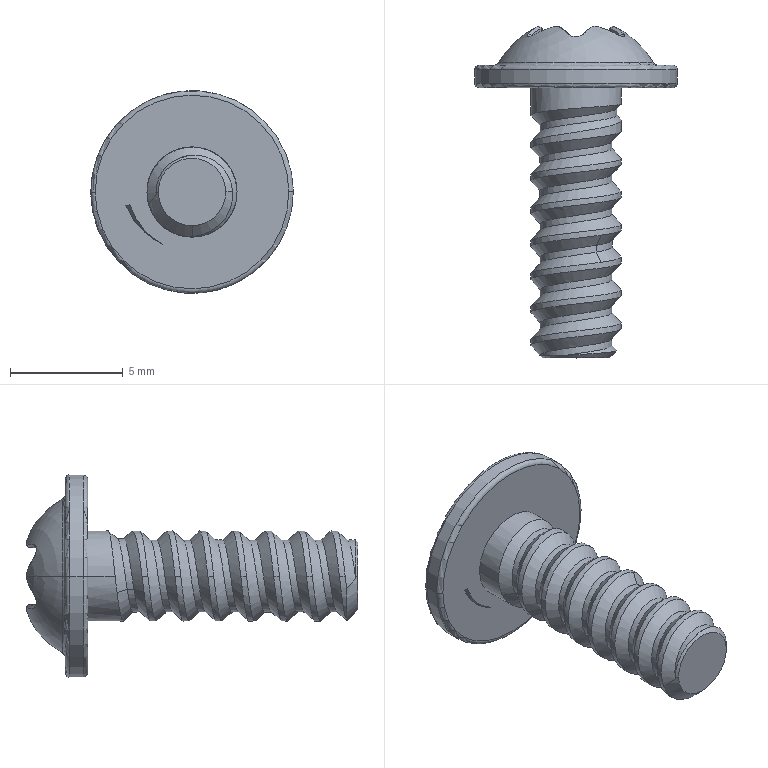Part | SolidWorks | features BaseBody 1 | 1 solid | 98 faces | box 9 x 14.741 x 9 mm | volume 214.18 mm3 | cylinder 30 | spline 25 | cone 17 | plane 16 | torus 6 | sphere 4 | commonest cylinder face diameters 4 x16 0.6 x12 9 x2